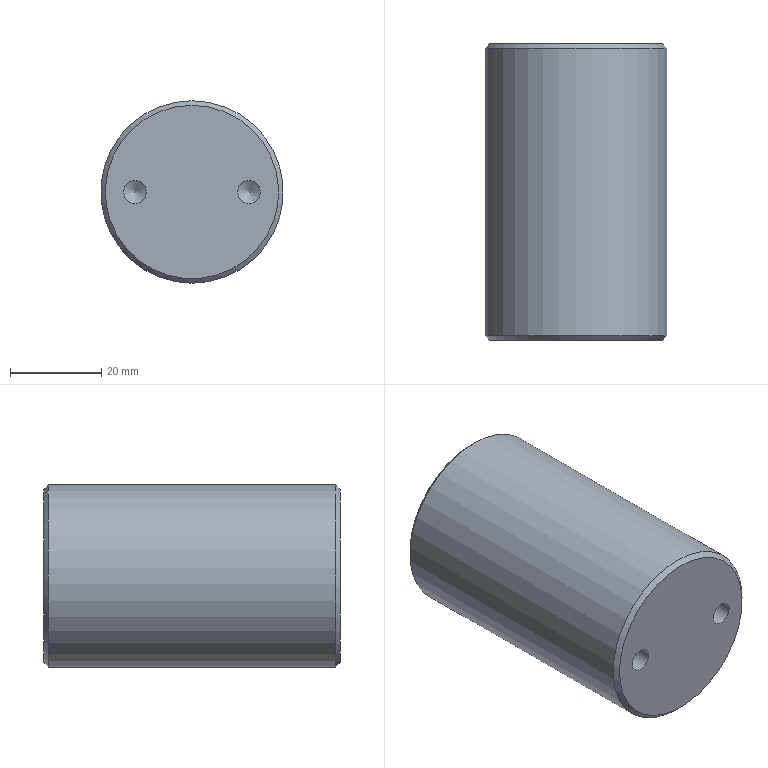Part | NX | 1 solid | 13 faces | box 40 x 65 x 40 mm | volume 80183 mm3 | cone 6 | cylinder 5 | plane 2 | commonest cylinder face diameters 5 x4 40 x1
STEP:
#1=CARTESIAN_POINT('',(0.,-31.5,20.));
#2=VERTEX_POINT('',#1);
#3=CARTESIAN_POINT('',(0.,-31.5,0.));
#4=DIRECTION('',(0.,1.,0.));
#5=DIRECTION('',(0.,0.,1.));
#6=AXIS2_PLACEMENT_3D('',#3,#4,#5);
#7=CIRCLE('',#6,20.);
#8=EDGE_CURVE('',#2,#2,#7,.T.);
#9=ORIENTED_EDGE('',*,*,#8,.T.);
#10=EDGE_LOOP('',(#9));
#11=FACE_BOUND('',#10,.T.);
#12=CARTESIAN_POINT('',(0.,31.5,20.));
#13=VERTEX_POINT('',#12);
#14=CARTESIAN_POINT('',(0.,31.5,0.));
#15=DIRECTION('',(0.,1.,0.));
#16=DIRECTION('',(0.,0.,1.));
#17=AXIS2_PLACEMENT_3D('',#14,#15,#16);
#18=CIRCLE('',#17,20.);
#19=EDGE_CURVE('',#13,#13,#18,.F.);
#20=ORIENTED_EDGE('',*,*,#19,.T.);
#21=EDGE_LOOP('',(#20));
#22=FACE_BOUND('',#21,.T.);
#23=CARTESIAN_POINT('',(0.,32.5,0.));
#24=DIRECTION('',(0.,-1.,0.));
#25=DIRECTION('',(0.,0.,-1.));
#26=AXIS2_PLACEMENT_3D('',#23,#24,#25);
#27=CYLINDRICAL_SURFACE('',#26,20.);
#28=ADVANCED_FACE('',(#11,#22),#27,.T.);
#29=CARTESIAN_POINT('',(0.,32.5,19.));
#30=VERTEX_POINT('',#29);
#31=CARTESIAN_POINT('',(0.,32.5,0.));
#32=DIRECTION('',(0.,1.,0.));
#33=DIRECTION('',(0.,0.,1.));
#34=AXIS2_PLACEMENT_3D('',#31,#32,#33);
#35=CIRCLE('',#34,19.);
#36=EDGE_CURVE('',#30,#30,#35,.T.);
#37=ORIENTED_EDGE('',*,*,#36,.T.);
#38=EDGE_LOOP('',(#37));
#39=FACE_BOUND('',#38,.T.);
#40=CARTESIAN_POINT('',(12.5,32.5,2.5));
#41=VERTEX_POINT('',#40);
#42=CARTESIAN_POINT('',(12.5,32.5,0.));
#43=DIRECTION('',(0.,1.,0.));
#44=DIRECTION('',(0.,0.,1.));
#45=AXIS2_PLACEMENT_3D('',#42,#43,#44);
#46=CIRCLE('',#45,2.5);
#47=EDGE_CURVE('',#41,#41,#46,.T.);
#48=ORIENTED_EDGE('',*,*,#47,.F.);
#49=EDGE_LOOP('',(#48));
#50=FACE_BOUND('',#49,.T.);
#51=CARTESIAN_POINT('',(-12.5,32.5,2.5));
#52=VERTEX_POINT('',#51);
#53=CARTESIAN_POINT('',(-12.5,32.5,0.));
#54=DIRECTION('',(0.,1.,0.));
#55=DIRECTION('',(0.,0.,1.));
#56=AXIS2_PLACEMENT_3D('',#53,#54,#55);
#57=CIRCLE('',#56,2.5);
#58=EDGE_CURVE('',#52,#52,#57,.T.);
#59=ORIENTED_EDGE('',*,*,#58,.F.);
#60=EDGE_LOOP('',(#59));
#61=FACE_BOUND('',#60,.T.);
#62=CARTESIAN_POINT('',(0.,32.5,0.));
#63=DIRECTION('',(0.,1.,0.));
#64=DIRECTION('',(0.,0.,1.));
#65=AXIS2_PLACEMENT_3D('',#62,#63,#64);
#66=PLANE('',#65);
#67=ADVANCED_FACE('',(#39,#50,#61),#66,.T.);
#68=CARTESIAN_POINT('',(12.5,-32.5,-2.5));
#69=VERTEX_POINT('',#68);
#70=CARTESIAN_POINT('',(12.5,-32.5,0.));
#71=DIRECTION('',(0.,-1.,0.));
#72=DIRECTION('',(0.,0.,-1.));
#73=AXIS2_PLACEMENT_3D('',#70,#71,#72);
#74=CIRCLE('',#73,2.5);
#75=EDGE_CURVE('',#69,#69,#74,.T.);
#76=ORIENTED_EDGE('',*,*,#75,.F.);
#77=EDGE_LOOP('',(#76));
#78=FACE_BOUND('',#77,.T.);
#79=CARTESIAN_POINT('',(-12.5,-32.5,-2.5));
#80=VERTEX_POINT('',#79);
#81=CARTESIAN_POINT('',(-12.5,-32.5,0.));
#82=DIRECTION('',(0.,-1.,0.));
#83=DIRECTION('',(0.,0.,-1.));
#84=AXIS2_PLACEMENT_3D('',#81,#82,#83);
#85=CIRCLE('',#84,2.5);
#86=EDGE_CURVE('',#80,#80,#85,.T.);
#87=ORIENTED_EDGE('',*,*,#86,.F.);
#88=EDGE_LOOP('',(#87));
#89=FACE_BOUND('',#88,.T.);
#90=CARTESIAN_POINT('',(0.,-32.5,19.));
#91=VERTEX_POINT('',#90);
#92=CARTESIAN_POINT('',(0.,-32.5,0.));
#93=DIRECTION('',(0.,1.,0.));
#94=DIRECTION('',(0.,0.,1.));
#95=AXIS2_PLACEMENT_3D('',#92,#93,#94);
#96=CIRCLE('',#95,19.);
#97=EDGE_CURVE('',#91,#91,#96,.F.);
#98=ORIENTED_EDGE('',*,*,#97,.T.);
#99=EDGE_LOOP('',(#98));
#100=FACE_BOUND('',#99,.T.);
#101=CARTESIAN_POINT('',(0.,-32.5,0.));
#102=DIRECTION('',(0.,1.,0.));
#103=DIRECTION('',(0.,0.,1.));
#104=AXIS2_PLACEMENT_3D('',#101,#102,#103);
#105=PLANE('',#104);
#106=ADVANCED_FACE('',(#78,#89,#100),#105,.F.);
#107=CARTESIAN_POINT('',(-12.5,13.998,0.));
#108=VERTEX_POINT('',#107);
#109=VERTEX_LOOP('',#108);
#110=FACE_BOUND('',#109,.T.);
#111=CARTESIAN_POINT('',(-12.5,15.5,2.5));
#112=VERTEX_POINT('',#111);
#113=CARTESIAN_POINT('',(-12.5,15.5,0.));
#114=DIRECTION('',(0.,1.,0.));
#115=DIRECTION('',(0.,0.,1.));
#116=AXIS2_PLACEMENT_3D('',#113,#114,#115);
#117=CIRCLE('',#116,2.5);
#118=EDGE_CURVE('',#112,#112,#117,.T.);
#119=ORIENTED_EDGE('',*,*,#118,.T.);
#120=EDGE_LOOP('',(#119));
#121=FACE_BOUND('',#120,.T.);
#122=CARTESIAN_POINT('',(-12.5,15.5,0.));
#123=DIRECTION('',(0.,1.,0.));
#124=DIRECTION('',(0.,0.,1.));
#125=AXIS2_PLACEMENT_3D('',#122,#123,#124);
#126=CONICAL_SURFACE('',#125,2.5,1.03);
#127=ADVANCED_FACE('',(#110,#121),#126,.F.);
#128=ORIENTED_EDGE('',*,*,#118,.F.);
#129=EDGE_LOOP('',(#128));
#130=FACE_BOUND('',#129,.T.);
#131=ORIENTED_EDGE('',*,*,#58,.T.);
#132=EDGE_LOOP('',(#131));
#133=FACE_BOUND('',#132,.T.);
#134=CARTESIAN_POINT('',(-12.5,32.5,0.));
#135=DIRECTION('',(0.,1.,0.));
#136=DIRECTION('',(0.,0.,1.));
#137=AXIS2_PLACEMENT_3D('',#134,#135,#136);
#138=CYLINDRICAL_SURFACE('',#137,2.5);
#139=ADVANCED_FACE('',(#130,#133),#138,.F.);
#140=CARTESIAN_POINT('',(12.5,13.998,0.));
#141=VERTEX_POINT('',#140);
#142=VERTEX_LOOP('',#141);
#143=FACE_BOUND('',#142,.T.);
#144=CARTESIAN_POINT('',(12.5,15.5,2.5));
#145=VERTEX_POINT('',#144);
#146=CARTESIAN_POINT('',(12.5,15.5,0.));
#147=DIRECTION('',(0.,1.,0.));
#148=DIRECTION('',(0.,0.,1.));
#149=AXIS2_PLACEMENT_3D('',#146,#147,#148);
#150=CIRCLE('',#149,2.5);
#151=EDGE_CURVE('',#145,#145,#150,.T.);
#152=ORIENTED_EDGE('',*,*,#151,.T.);
#153=EDGE_LOOP('',(#152));
#154=FACE_BOUND('',#153,.T.);
#155=CARTESIAN_POINT('',(12.5,15.5,0.));
#156=DIRECTION('',(0.,1.,0.));
#157=DIRECTION('',(0.,0.,1.));
#158=AXIS2_PLACEMENT_3D('',#155,#156,#157);
#159=CONICAL_SURFACE('',#158,2.5,1.03);
#160=ADVANCED_FACE('',(#143,#154),#159,.F.);
#161=ORIENTED_EDGE('',*,*,#151,.F.);
#162=EDGE_LOOP('',(#161));
#163=FACE_BOUND('',#162,.T.);
#164=ORIENTED_EDGE('',*,*,#47,.T.);
#165=EDGE_LOOP('',(#164));
#166=FACE_BOUND('',#165,.T.);
#167=CARTESIAN_POINT('',(12.5,32.5,0.));
#168=DIRECTION('',(0.,1.,0.));
#169=DIRECTION('',(0.,0.,1.));
#170=AXIS2_PLACEMENT_3D('',#167,#168,#169);
#171=CYLINDRICAL_SURFACE('',#170,2.5);
#172=ADVANCED_FACE('',(#163,#166),#171,.F.);
#173=ORIENTED_EDGE('',*,*,#97,.F.);
#174=EDGE_LOOP('',(#173));
#175=FACE_BOUND('',#174,.T.);
#176=ORIENTED_EDGE('',*,*,#8,.F.);
#177=EDGE_LOOP('',(#176));
#178=FACE_BOUND('',#177,.T.);
#179=CARTESIAN_POINT('',(0.,-31.5,0.));
#180=DIRECTION('',(0.,1.,0.));
#181=DIRECTION('',(0.,0.,1.));
#182=AXIS2_PLACEMENT_3D('',#179,#180,#181);
#183=CONICAL_SURFACE('',#182,20.,0.7854);
#184=ADVANCED_FACE('',(#175,#178),#183,.T.);
#185=ORIENTED_EDGE('',*,*,#19,.F.);
#186=EDGE_LOOP('',(#185));
#187=FACE_BOUND('',#186,.T.);
#188=ORIENTED_EDGE('',*,*,#36,.F.);
#189=EDGE_LOOP('',(#188));
#190=FACE_BOUND('',#189,.T.);
#191=CARTESIAN_POINT('',(0.,32.5,0.));
#192=DIRECTION('',(0.,-1.,0.));
#193=DIRECTION('',(0.,0.,-1.));
#194=AXIS2_PLACEMENT_3D('',#191,#192,#193);
#195=CONICAL_SURFACE('',#194,19.,0.7854);
#196=ADVANCED_FACE('',(#187,#190),#195,.T.);
#197=CARTESIAN_POINT('',(-12.5,-13.998,0.));
#198=VERTEX_POINT('',#197);
#199=VERTEX_LOOP('',#198);
#200=FACE_BOUND('',#199,.T.);
#201=CARTESIAN_POINT('',(-12.5,-15.5,-2.5));
#202=VERTEX_POINT('',#201);
#203=CARTESIAN_POINT('',(-12.5,-15.5,0.));
#204=DIRECTION('',(0.,-1.,0.));
#205=DIRECTION('',(0.,0.,-1.));
#206=AXIS2_PLACEMENT_3D('',#203,#204,#205);
#207=CIRCLE('',#206,2.5);
#208=EDGE_CURVE('',#202,#202,#207,.T.);
#209=ORIENTED_EDGE('',*,*,#208,.T.);
#210=EDGE_LOOP('',(#209));
#211=FACE_BOUND('',#210,.T.);
#212=CARTESIAN_POINT('',(-12.5,-15.5,0.));
#213=DIRECTION('',(0.,-1.,0.));
#214=DIRECTION('',(0.,0.,-1.));
#215=AXIS2_PLACEMENT_3D('',#212,#213,#214);
#216=CONICAL_SURFACE('',#215,2.5,1.03);
#217=ADVANCED_FACE('',(#200,#211),#216,.F.);
#218=ORIENTED_EDGE('',*,*,#208,.F.);
#219=EDGE_LOOP('',(#218));
#220=FACE_BOUND('',#219,.T.);
#221=ORIENTED_EDGE('',*,*,#86,.T.);
#222=EDGE_LOOP('',(#221));
#223=FACE_BOUND('',#222,.T.);
#224=CARTESIAN_POINT('',(-12.5,-32.5,0.));
#225=DIRECTION('',(0.,-1.,0.));
#226=DIRECTION('',(0.,0.,-1.));
#227=AXIS2_PLACEMENT_3D('',#224,#225,#226);
#228=CYLINDRICAL_SURFACE('',#227,2.5);
#229=ADVANCED_FACE('',(#220,#223),#228,.F.);
#230=CARTESIAN_POINT('',(12.5,-13.998,0.));
#231=VERTEX_POINT('',#230);
#232=VERTEX_LOOP('',#231);
#233=FACE_BOUND('',#232,.T.);
#234=CARTESIAN_POINT('',(12.5,-15.5,-2.5));
#235=VERTEX_POINT('',#234);
#236=CARTESIAN_POINT('',(12.5,-15.5,0.));
#237=DIRECTION('',(0.,-1.,0.));
#238=DIRECTION('',(0.,0.,-1.));
#239=AXIS2_PLACEMENT_3D('',#236,#237,#238);
#240=CIRCLE('',#239,2.5);
#241=EDGE_CURVE('',#235,#235,#240,.T.);
#242=ORIENTED_EDGE('',*,*,#241,.T.);
#243=EDGE_LOOP('',(#242));
#244=FACE_BOUND('',#243,.T.);
#245=CARTESIAN_POINT('',(12.5,-15.5,0.));
#246=DIRECTION('',(0.,-1.,0.));
#247=DIRECTION('',(0.,0.,-1.));
#248=AXIS2_PLACEMENT_3D('',#245,#246,#247);
#249=CONICAL_SURFACE('',#248,2.5,1.03);
#250=ADVANCED_FACE('',(#233,#244),#249,.F.);
#251=ORIENTED_EDGE('',*,*,#241,.F.);
#252=EDGE_LOOP('',(#251));
#253=FACE_BOUND('',#252,.T.);
#254=ORIENTED_EDGE('',*,*,#75,.T.);
#255=EDGE_LOOP('',(#254));
#256=FACE_BOUND('',#255,.T.);
#257=CARTESIAN_POINT('',(12.5,-32.5,0.));
#258=DIRECTION('',(0.,-1.,0.));
#259=DIRECTION('',(0.,0.,-1.));
#260=AXIS2_PLACEMENT_3D('',#257,#258,#259);
#261=CYLINDRICAL_SURFACE('',#260,2.5);
#262=ADVANCED_FACE('',(#253,#256),#261,.F.);
#263=CLOSED_SHELL('',(#28,#67,#106,#127,#139,#160,#172,#184,#196,#217,#229,#250,#262));
#264=MANIFOLD_SOLID_BREP('',#263);
#265=(LENGTH_UNIT()NAMED_UNIT(*)SI_UNIT(.MILLI.,.METRE.));
#266=UNCERTAINTY_MEASURE_WITH_UNIT(LENGTH_MEASURE(0.00001),#265,'','');
#267=(NAMED_UNIT(*)PLANE_ANGLE_UNIT()SI_UNIT($,.RADIAN.));
#268=(NAMED_UNIT(*)SI_UNIT($,.STERADIAN.)SOLID_ANGLE_UNIT());
#269=(GEOMETRIC_REPRESENTATION_CONTEXT(3)GLOBAL_UNCERTAINTY_ASSIGNED_CONTEXT((#266))GLOBAL_UNIT_ASSIGNED_CONTEXT((#265,#267,#268))REPRESENTATION_CONTEXT('',''));
#270=ADVANCED_BREP_SHAPE_REPRESENTATION('',(#264),#269);